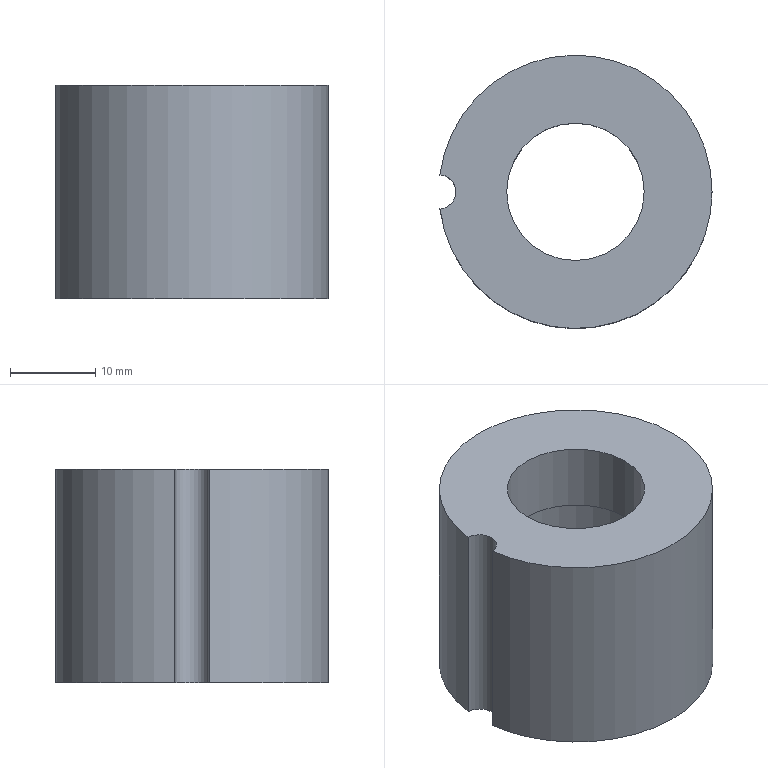Part | NX | features solid 2 | 1 solid | 7 faces | box 31.875 x 32 x 25 mm | volume 12659 mm3 | cylinder 4 | plane 3 | commonest cylinder face diameters 4 x1 16.1 x1 20.6 x1 32 x1
STEP:
#1=CARTESIAN_POINT('',(-639.372,-423.86,21.));
#2=VERTEX_POINT('',#1);
#3=CARTESIAN_POINT('',(-639.372,-423.86,46.));
#4=VERTEX_POINT('',#3);
#5=CARTESIAN_POINT('',(-639.372,-423.86,33.5));
#6=DIRECTION('',(0.,0.,1.));
#7=VECTOR('',#6,1000.);
#8=LINE('',#5,#7);
#9=EDGE_CURVE('',#2,#4,#8,.T.);
#10=ORIENTED_EDGE('',*,*,#9,.T.);
#11=CARTESIAN_POINT('',(-639.372,-427.852,46.));
#12=VERTEX_POINT('',#11);
#13=CARTESIAN_POINT('',(-623.497,-425.856,46.));
#14=DIRECTION('',(0.,0.,-1.));
#15=DIRECTION('',(-1.,0.,0.));
#16=AXIS2_PLACEMENT_3D('',#13,#14,#15);
#17=CIRCLE('',#16,16.);
#18=EDGE_CURVE('',#4,#12,#17,.T.);
#19=ORIENTED_EDGE('',*,*,#18,.T.);
#20=CARTESIAN_POINT('',(-639.372,-427.852,21.));
#21=VERTEX_POINT('',#20);
#22=CARTESIAN_POINT('',(-639.372,-427.852,33.5));
#23=DIRECTION('',(0.,0.,1.));
#24=VECTOR('',#23,1000.);
#25=LINE('',#22,#24);
#26=EDGE_CURVE('',#12,#21,#25,.F.);
#27=ORIENTED_EDGE('',*,*,#26,.T.);
#28=CARTESIAN_POINT('',(-623.497,-425.856,21.));
#29=DIRECTION('',(0.,0.,-1.));
#30=DIRECTION('',(-1.,0.,0.));
#31=AXIS2_PLACEMENT_3D('',#28,#29,#30);
#32=CIRCLE('',#31,16.);
#33=EDGE_CURVE('',#2,#21,#32,.T.);
#34=ORIENTED_EDGE('',*,*,#33,.F.);
#35=EDGE_LOOP('',(#10,#19,#27,#34));
#36=FACE_BOUND('',#35,.T.);
#37=CARTESIAN_POINT('',(-623.497,-425.856,21.));
#38=DIRECTION('',(0.,0.,1.));
#39=DIRECTION('',(-1.,0.,0.));
#40=AXIS2_PLACEMENT_3D('',#37,#38,#39);
#41=CYLINDRICAL_SURFACE('',#40,16.);
#42=ADVANCED_FACE('',(#36),#41,.T.);
#43=CARTESIAN_POINT('',(-633.797,-425.856,21.));
#44=VERTEX_POINT('',#43);
#45=CARTESIAN_POINT('',(-623.497,-425.856,21.));
#46=DIRECTION('',(0.,0.,-1.));
#47=DIRECTION('',(-1.,0.,0.));
#48=AXIS2_PLACEMENT_3D('',#45,#46,#47);
#49=CIRCLE('',#48,10.3);
#50=EDGE_CURVE('',#44,#44,#49,.T.);
#51=ORIENTED_EDGE('',*,*,#50,.F.);
#52=EDGE_LOOP('',(#51));
#53=FACE_BOUND('',#52,.T.);
#54=ORIENTED_EDGE('',*,*,#33,.T.);
#55=CARTESIAN_POINT('',(-639.497,-425.856,21.));
#56=DIRECTION('',(0.,0.,-1.));
#57=DIRECTION('',(-1.,0.,0.));
#58=AXIS2_PLACEMENT_3D('',#55,#56,#57);
#59=CIRCLE('',#58,2.);
#60=EDGE_CURVE('',#2,#21,#59,.T.);
#61=ORIENTED_EDGE('',*,*,#60,.F.);
#62=EDGE_LOOP('',(#54,#61));
#63=FACE_BOUND('',#62,.T.);
#64=CARTESIAN_POINT('',(-623.497,-425.856,21.));
#65=DIRECTION('',(0.,0.,1.));
#66=DIRECTION('',(-1.,0.,0.));
#67=AXIS2_PLACEMENT_3D('',#64,#65,#66);
#68=PLANE('',#67);
#69=ADVANCED_FACE('',(#53,#63),#68,.F.);
#70=CARTESIAN_POINT('',(-631.547,-425.856,46.));
#71=VERTEX_POINT('',#70);
#72=CARTESIAN_POINT('',(-623.497,-425.856,46.));
#73=DIRECTION('',(0.,0.,-1.));
#74=DIRECTION('',(-1.,0.,0.));
#75=AXIS2_PLACEMENT_3D('',#72,#73,#74);
#76=CIRCLE('',#75,8.05);
#77=EDGE_CURVE('',#71,#71,#76,.T.);
#78=ORIENTED_EDGE('',*,*,#77,.T.);
#79=EDGE_LOOP('',(#78));
#80=FACE_BOUND('',#79,.T.);
#81=CARTESIAN_POINT('',(-639.497,-425.856,46.));
#82=DIRECTION('',(0.,0.,-1.));
#83=DIRECTION('',(-1.,0.,0.));
#84=AXIS2_PLACEMENT_3D('',#81,#82,#83);
#85=CIRCLE('',#84,2.);
#86=EDGE_CURVE('',#4,#12,#85,.T.);
#87=ORIENTED_EDGE('',*,*,#86,.T.);
#88=ORIENTED_EDGE('',*,*,#18,.F.);
#89=EDGE_LOOP('',(#87,#88));
#90=FACE_BOUND('',#89,.T.);
#91=CARTESIAN_POINT('',(-623.497,-425.856,46.));
#92=DIRECTION('',(0.,0.,1.));
#93=DIRECTION('',(-1.,0.,0.));
#94=AXIS2_PLACEMENT_3D('',#91,#92,#93);
#95=PLANE('',#94);
#96=ADVANCED_FACE('',(#80,#90),#95,.T.);
#97=ORIENTED_EDGE('',*,*,#50,.T.);
#98=EDGE_LOOP('',(#97));
#99=FACE_BOUND('',#98,.T.);
#100=CARTESIAN_POINT('',(-633.797,-425.856,38.));
#101=VERTEX_POINT('',#100);
#102=CARTESIAN_POINT('',(-623.497,-425.856,38.));
#103=DIRECTION('',(0.,0.,-1.));
#104=DIRECTION('',(-1.,0.,0.));
#105=AXIS2_PLACEMENT_3D('',#102,#103,#104);
#106=CIRCLE('',#105,10.3);
#107=EDGE_CURVE('',#101,#101,#106,.T.);
#108=ORIENTED_EDGE('',*,*,#107,.F.);
#109=EDGE_LOOP('',(#108));
#110=FACE_BOUND('',#109,.T.);
#111=CARTESIAN_POINT('',(-623.497,-425.856,21.));
#112=DIRECTION('',(0.,0.,1.));
#113=DIRECTION('',(-1.,0.,0.));
#114=AXIS2_PLACEMENT_3D('',#111,#112,#113);
#115=CYLINDRICAL_SURFACE('',#114,10.3);
#116=ADVANCED_FACE('',(#99,#110),#115,.F.);
#117=CARTESIAN_POINT('',(-631.547,-425.856,38.));
#118=VERTEX_POINT('',#117);
#119=CARTESIAN_POINT('',(-623.497,-425.856,38.));
#120=DIRECTION('',(0.,0.,-1.));
#121=DIRECTION('',(-1.,0.,0.));
#122=AXIS2_PLACEMENT_3D('',#119,#120,#121);
#123=CIRCLE('',#122,8.05);
#124=EDGE_CURVE('',#118,#118,#123,.T.);
#125=ORIENTED_EDGE('',*,*,#124,.F.);
#126=EDGE_LOOP('',(#125));
#127=FACE_BOUND('',#126,.T.);
#128=ORIENTED_EDGE('',*,*,#107,.T.);
#129=EDGE_LOOP('',(#128));
#130=FACE_BOUND('',#129,.T.);
#131=CARTESIAN_POINT('',(-623.497,-425.856,38.));
#132=DIRECTION('',(0.,0.,1.));
#133=DIRECTION('',(-1.,0.,0.));
#134=AXIS2_PLACEMENT_3D('',#131,#132,#133);
#135=PLANE('',#134);
#136=ADVANCED_FACE('',(#127,#130),#135,.F.);
#137=ORIENTED_EDGE('',*,*,#9,.F.);
#138=ORIENTED_EDGE('',*,*,#60,.T.);
#139=ORIENTED_EDGE('',*,*,#26,.F.);
#140=ORIENTED_EDGE('',*,*,#86,.F.);
#141=EDGE_LOOP('',(#137,#138,#139,#140));
#142=FACE_BOUND('',#141,.T.);
#143=CARTESIAN_POINT('',(-639.497,-425.856,21.));
#144=DIRECTION('',(0.,0.,1.));
#145=DIRECTION('',(-1.,0.,0.));
#146=AXIS2_PLACEMENT_3D('',#143,#144,#145);
#147=CYLINDRICAL_SURFACE('',#146,2.);
#148=ADVANCED_FACE('',(#142),#147,.F.);
#149=ORIENTED_EDGE('',*,*,#77,.F.);
#150=EDGE_LOOP('',(#149));
#151=FACE_BOUND('',#150,.T.);
#152=ORIENTED_EDGE('',*,*,#124,.T.);
#153=EDGE_LOOP('',(#152));
#154=FACE_BOUND('',#153,.T.);
#155=CARTESIAN_POINT('',(-623.497,-425.856,21.));
#156=DIRECTION('',(0.,0.,1.));
#157=DIRECTION('',(-1.,0.,0.));
#158=AXIS2_PLACEMENT_3D('',#155,#156,#157);
#159=CYLINDRICAL_SURFACE('',#158,8.05);
#160=ADVANCED_FACE('',(#151,#154),#159,.F.);
#161=CLOSED_SHELL('',(#42,#69,#96,#116,#136,#148,#160));
#162=MANIFOLD_SOLID_BREP('',#161);
#163=(LENGTH_UNIT()NAMED_UNIT(*)SI_UNIT(.MILLI.,.METRE.));
#164=UNCERTAINTY_MEASURE_WITH_UNIT(LENGTH_MEASURE(0.00001),#163,'','');
#165=(NAMED_UNIT(*)PLANE_ANGLE_UNIT()SI_UNIT($,.RADIAN.));
#166=(NAMED_UNIT(*)SI_UNIT($,.STERADIAN.)SOLID_ANGLE_UNIT());
#167=(GEOMETRIC_REPRESENTATION_CONTEXT(3)GLOBAL_UNCERTAINTY_ASSIGNED_CONTEXT((#164))GLOBAL_UNIT_ASSIGNED_CONTEXT((#163,#165,#166))REPRESENTATION_CONTEXT('',''));
#168=ADVANCED_BREP_SHAPE_REPRESENTATION('',(#162),#167);